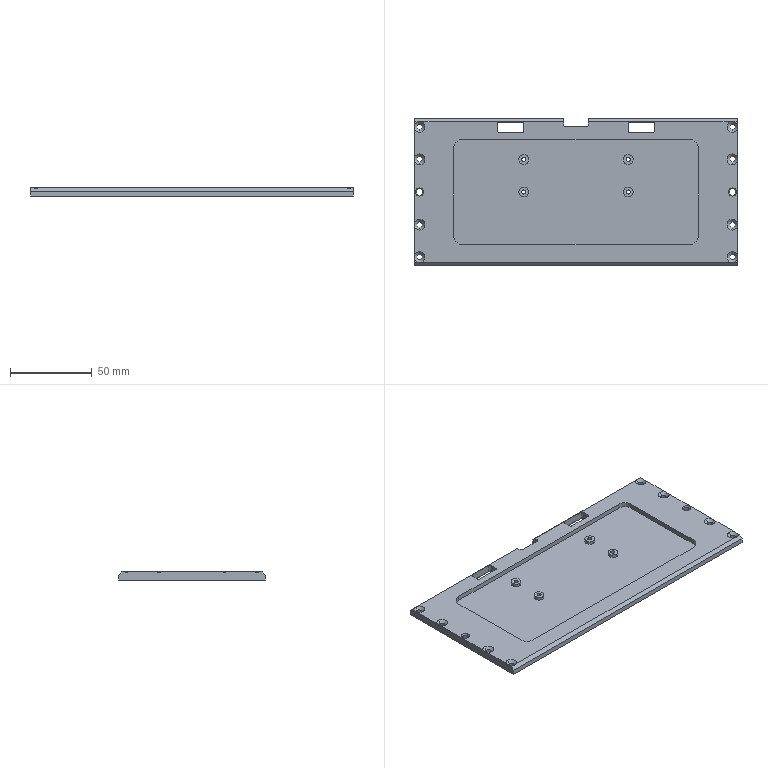NC program | NX | posted with a generic post | part box 198 x 90 x 5 mm
Lines 7363 to 7766 of 7766:
(CUTTERCOMP17 , TOOL : D2)
N14634 T17 M6
N14636 G54
N14638 G17 G0 G90 X-96. Y0. S9500 M3
N14640 G43 Z30. H17
N14642 Z0.5
N14644 G41 G94 G1 X-95.996 Y-0.1 F1100. D17
N14646 G3 X-95.05 Y0. R0.478
N14648 X-95.05 Y0. Z-1.5 I-0.95 J0.
N14650 X-95.05 Y0. Z-3.5 I-0.95 J0.
N14652 X-96. Y-0.95 Z-5. R-0.95
N14654 X-95.05 Y0. R0.95
N14656 X-96. Y-0.95 R-0.95
N14658 X-95.9 Y-0.004 R0.478
N14660 G40
N14662 G1 X-96. Y0.
N14664 G0 Z30.
N14666 X96.
N14668 Z0.5
N14670 G41 G1 X96.004 Y-0.1
N14672 G3 X96.95 Y0. R0.478
N14674 X96.95 Y0. Z-1.5 I-0.95 J0.
N14676 X96.95 Y0. Z-3.5 I-0.95 J0.
N14678 X96. Y-0.95 Z-5. R-0.95
N14680 X96.95 Y0. R0.95
N14682 X96. Y-0.95 R-0.95
N14684 X96.1 Y-0.004 R0.478
N14686 G40
N14688 G1 X96. Y0.
N14690 G0 Z30.
N14692 M5
(ZLEVEL_PROFILE_COPY_1_COPY_COPY_1 , TOOL : D10JING)
N14694 T14 M6
N14696 G54
N14698 G17 G0 G90 X100.622 Y-51.809 S9500 M3
N14700 G43 Z30. H14
N14702 Z-3.525
N14704 G94 G1 Z-4.525 F1000.
N14706 X99.866 Y-50.5
N14708 G3 X99. Y-50. R1.
N14710 G1 X-99. F1200.
N14712 G2 X-104. Y-45. R5.
N14714 G1 Y45.
N14716 G2 X-99. Y50. R5.
N14718 G1 X-7.5
N14720 G2 X-2.5 Y45. R5.
N14722 G1 X2.5
N14724 G2 X7.5 Y50. R5.
N14726 G1 X99.
N14728 G2 X104. Y45. R5.
N14730 G1 Y-45.
N14732 G2 X99. Y-50. R5.
N14734 G1 X-99. Z-4.565
N14736 X-99.49 Y-49.976
N14738 X-99.975 Y-49.904 Z-4.566
N14740 X-100.451 Y-49.785
N14742 X-100.913 Y-49.619
N14744 X-101.357 Y-49.41
N14746 X-101.778 Y-49.157
N14748 X-102.172 Y-48.865
N14750 X-102.536 Y-48.536
N14752 X-102.865 Y-48.172
N14754 X-103.157 Y-47.778
N14756 X-103.41 Y-47.357
N14758 X-103.619 Y-46.913 Z-4.567
N14760 X-103.785 Y-46.451
N14762 X-103.904 Y-45.975
N14764 X-103.976 Y-45.49
N14766 X-104. Y-45.
N14768 X-104.003 Y-40. Z-4.568
N14770 X-104. Y-35. Z-4.569
N14772 Y35. Z-4.583
N14774 X-104.003 Y40. Z-4.584
N14776 X-104. Y45. Z-4.585
N14778 X-103.976 Y45.49
N14780 X-103.904 Y45.975 Z-4.586
N14782 X-103.785 Y46.451
N14784 X-103.619 Y46.913
N14786 X-103.41 Y47.357
N14788 X-103.157 Y47.778
N14790 X-102.865 Y48.172
N14792 X-102.536 Y48.536
N14794 X-102.172 Y48.865
N14796 X-101.778 Y49.157
N14798 X-101.357 Y49.41
N14800 X-100.913 Y49.619 Z-4.587
N14802 X-100.451 Y49.785
N14804 X-99.975 Y49.904
N14806 X-99.49 Y49.976
N14808 X-99. Y50.
N14810 X-7.5 Z-4.606
N14812 X-7.01 Y49.976
N14814 X-6.525 Y49.904
N14816 X-6.049 Y49.785
N14818 X-5.587 Y49.619
N14820 X-5.143 Y49.41
N14822 X-4.722 Y49.157
N14824 X-4.328 Y48.865
N14826 X-3.964 Y48.536
N14828 X-3.635 Y48.172
N14830 X-3.343 Y47.778 Z-4.607
N14832 X-3.09 Y47.357
N14834 X-2.881 Y46.913
N14836 X-2.715 Y46.451
N14838 X-2.596 Y45.975
N14840 X-2.525 Y45.5
N14842 X-2.5 Y45.
N14844 X2.5 Z-4.608
N14846 X2.525 Y45.5
N14848 X2.596 Y45.975
N14850 X2.715 Y46.451
N14852 X2.881 Y46.913 Z-4.609
N14854 X3.09 Y47.357
N14856 X3.343 Y47.778
N14858 X3.635 Y48.172
N14860 X3.964 Y48.536
N14862 X4.328 Y48.865
N14864 X4.722 Y49.157
N14866 X5.143 Y49.41
N14868 X5.587 Y49.619
N14870 X6.049 Y49.785
N14872 X6.525 Y49.904 Z-4.61
N14874 X7.01 Y49.976
N14876 X7.5 Y50.
N14878 X99. Z-4.628
N14880 X99.49 Y49.976 Z-4.629
N14882 X99.975 Y49.904
N14884 X100.451 Y49.785
N14886 X100.913 Y49.619
N14888 X101.357 Y49.41
N14890 X101.778 Y49.157
N14892 X102.172 Y48.865
N14894 X102.536 Y48.536
N14896 X102.865 Y48.172
N14898 X103.157 Y47.778
N14900 X103.41 Y47.357 Z-4.63
N14902 X103.619 Y46.913
N14904 X103.785 Y46.451
N14906 X103.904 Y45.975
N14908 X103.976 Y45.49
N14910 X104. Y45.
N14912 X104.005 Y40.5 Z-4.631
N14914 X104. Y36. Z-4.632
N14916 Y-36. Z-4.647
N14918 X104.005 Y-40.5
N14920 X104. Y-45. Z-4.648
N14922 X103.976 Y-45.49 Z-4.649
N14924 X103.904 Y-45.975
N14926 X103.785 Y-46.451
N14928 X103.619 Y-46.913
N14930 X103.41 Y-47.357
N14932 X103.157 Y-47.778
N14934 X102.865 Y-48.172
N14936 X102.536 Y-48.536
N14938 X102.172 Y-48.865
N14940 X101.778 Y-49.157
N14942 X101.357 Y-49.41 Z-4.65
N14944 X100.913 Y-49.619
N14946 X100.451 Y-49.785
N14948 X99.975 Y-49.904
N14950 X99.49 Y-49.976
N14952 X99. Y-50.
N14954 X-99. Z-4.69
N14956 X-99.49 Y-49.976
N14958 X-99.975 Y-49.904 Z-4.691
N14960 X-100.451 Y-49.785
N14962 X-100.913 Y-49.619
N14964 X-101.357 Y-49.41
N14966 X-101.778 Y-49.157
N14968 X-102.172 Y-48.865
N14970 X-102.536 Y-48.536
N14972 X-102.865 Y-48.172
N14974 X-103.157 Y-47.778
N14976 X-103.41 Y-47.357
N14978 X-103.619 Y-46.913 Z-4.692
N14980 X-103.785 Y-46.451
N14982 X-103.904 Y-45.975
N14984 X-103.976 Y-45.49
N14986 X-104. Y-45.
N14988 X-104.003 Y-40. Z-4.693
N14990 X-104. Y-35. Z-4.694
N14992 Y35. Z-4.708
N14994 X-104.003 Y40. Z-4.709
N14996 X-104. Y45. Z-4.71
N14998 X-103.976 Y45.49
N15000 X-103.904 Y45.975 Z-4.711
N15002 X-103.785 Y46.451
N15004 X-103.619 Y46.913
N15006 X-103.41 Y47.357
N15008 X-103.157 Y47.778
N15010 X-102.865 Y48.172
N15012 X-102.536 Y48.536
N15014 X-102.172 Y48.865
N15016 X-101.778 Y49.157
N15018 X-101.357 Y49.41
N15020 X-100.913 Y49.619 Z-4.712
N15022 X-100.451 Y49.785
N15024 X-99.975 Y49.904
N15026 X-99.49 Y49.976
N15028 X-99. Y50.
N15030 X-7.5 Z-4.731
N15032 X-7.01 Y49.976
N15034 X-6.525 Y49.904
N15036 X-6.049 Y49.785
N15038 X-5.587 Y49.619
N15040 X-5.143 Y49.41
N15042 X-4.722 Y49.157
N15044 X-4.328 Y48.865
N15046 X-3.964 Y48.536
N15048 X-3.635 Y48.172
N15050 X-3.343 Y47.778 Z-4.732
N15052 X-3.09 Y47.357
N15054 X-2.881 Y46.913
N15056 X-2.715 Y46.451
N15058 X-2.596 Y45.975
N15060 X-2.525 Y45.5
N15062 X-2.5 Y45.
N15064 X2.5 Z-4.733
N15066 X2.525 Y45.5
N15068 X2.596 Y45.975
N15070 X2.715 Y46.451
N15072 X2.881 Y46.913 Z-4.734
N15074 X3.09 Y47.357
N15076 X3.343 Y47.778
N15078 X3.635 Y48.172
N15080 X3.964 Y48.536
N15082 X4.328 Y48.865
N15084 X4.722 Y49.157
N15086 X5.143 Y49.41
N15088 X5.587 Y49.619
N15090 X6.049 Y49.785
N15092 X6.525 Y49.904 Z-4.735
N15094 X7.01 Y49.976
N15096 X7.5 Y50.
N15098 X99. Z-4.753
N15100 X99.49 Y49.976 Z-4.754
N15102 X99.975 Y49.904
N15104 X100.451 Y49.785
N15106 X100.913 Y49.619
N15108 X101.357 Y49.41
N15110 X101.778 Y49.157
N15112 X102.172 Y48.865
N15114 X102.536 Y48.536
N15116 X102.865 Y48.172
N15118 X103.157 Y47.778
N15120 X103.41 Y47.357 Z-4.755
N15122 X103.619 Y46.913
N15124 X103.785 Y46.451
N15126 X103.904 Y45.975
N15128 X103.976 Y45.49
N15130 X104. Y45.
N15132 X104.005 Y40.5 Z-4.756
N15134 X104. Y36. Z-4.757
N15136 Y-36. Z-4.772
N15138 X104.005 Y-40.5
N15140 X104. Y-45. Z-4.773
N15142 X103.976 Y-45.49 Z-4.774
N15144 X103.904 Y-45.975
N15146 X103.785 Y-46.451
N15148 X103.619 Y-46.913
N15150 X103.41 Y-47.357
N15152 X103.157 Y-47.778
N15154 X102.865 Y-48.172
N15156 X102.536 Y-48.536
N15158 X102.172 Y-48.865
N15160 X101.778 Y-49.157
N15162 X101.357 Y-49.41 Z-4.775
N15164 X100.913 Y-49.619
N15166 X100.451 Y-49.785
N15168 X99.975 Y-49.904
N15170 X99.49 Y-49.976
N15172 X99. Y-50.
N15174 X-99. Z-4.815
N15176 X-99.49 Y-49.976
N15178 X-99.975 Y-49.904 Z-4.816
N15180 X-100.451 Y-49.785
N15182 X-100.913 Y-49.619
N15184 X-101.357 Y-49.41
N15186 X-101.778 Y-49.157
N15188 X-102.172 Y-48.865
N15190 X-102.536 Y-48.536
N15192 X-102.865 Y-48.172
N15194 X-103.157 Y-47.778
N15196 X-103.41 Y-47.357
N15198 X-103.619 Y-46.913 Z-4.817
N15200 X-103.785 Y-46.451
N15202 X-103.904 Y-45.975
N15204 X-103.976 Y-45.49
N15206 X-104. Y-45.
N15208 X-104.003 Y-40. Z-4.818
N15210 X-104. Y-35. Z-4.819
N15212 Y35. Z-4.833
N15214 X-104.003 Y40. Z-4.834
N15216 X-104. Y45. Z-4.835
N15218 X-103.976 Y45.49
N15220 X-103.904 Y45.975 Z-4.836
N15222 X-103.785 Y46.451
N15224 X-103.619 Y46.913
N15226 X-103.41 Y47.357
N15228 X-103.157 Y47.778
N15230 X-102.865 Y48.172
N15232 X-102.536 Y48.536
N15234 X-102.172 Y48.865
N15236 X-101.778 Y49.157
N15238 X-101.357 Y49.41
N15240 X-100.913 Y49.619 Z-4.837
N15242 X-100.451 Y49.785
N15244 X-99.975 Y49.904
N15246 X-99.49 Y49.976
N15248 X-99. Y50.
N15250 X-7.5 Z-4.856
N15252 X-7.01 Y49.976
N15254 X-6.525 Y49.904
N15256 X-6.049 Y49.785
N15258 X-5.587 Y49.619
N15260 X-5.143 Y49.41
N15262 X-4.722 Y49.157
N15264 X-4.328 Y48.865
N15266 X-3.964 Y48.536
N15268 X-3.635 Y48.172
N15270 X-3.343 Y47.778 Z-4.857
N15272 X-3.09 Y47.357
N15274 X-2.881 Y46.913
N15276 X-2.715 Y46.451
N15278 X-2.596 Y45.975
N15280 X-2.525 Y45.5
N15282 X-2.5 Y45.
N15284 X2.5 Z-4.858
N15286 X2.525 Y45.5
N15288 X2.596 Y45.975
N15290 X2.715 Y46.451
N15292 X2.881 Y46.913 Z-4.859
N15294 X3.09 Y47.357
N15296 X3.343 Y47.778
N15298 X3.635 Y48.172
N15300 X3.964 Y48.536
N15302 X4.328 Y48.865
N15304 X4.722 Y49.157
N15306 X5.143 Y49.41
N15308 X5.587 Y49.619
N15310 X6.049 Y49.785
N15312 X6.525 Y49.904 Z-4.86
N15314 X7.01 Y49.976
N15316 X7.5 Y50.
N15318 X99. Z-4.878
N15320 X99.49 Y49.976 Z-4.879
N15322 X99.975 Y49.904
N15324 X100.451 Y49.785
N15326 X100.913 Y49.619
N15328 X101.357 Y49.41
N15330 X101.778 Y49.157
N15332 X102.172 Y48.865
N15334 X102.536 Y48.536
N15336 X102.865 Y48.172
N15338 X103.157 Y47.778
N15340 X103.41 Y47.357 Z-4.88
N15342 X103.619 Y46.913
N15344 X103.785 Y46.451
N15346 X103.904 Y45.975
N15348 X103.976 Y45.49
N15350 X104. Y45.
N15352 X104.005 Y40.5 Z-4.881
N15354 X104. Y36. Z-4.882
N15356 Y-36. Z-4.897
N15358 X104.005 Y-40.5
N15360 X104. Y-45. Z-4.898
N15362 X103.976 Y-45.49 Z-4.899
N15364 X103.904 Y-45.975
N15366 X103.785 Y-46.451
N15368 X103.619 Y-46.913
N15370 X103.41 Y-47.357
N15372 X103.157 Y-47.778
N15374 X102.865 Y-48.172
N15376 X102.536 Y-48.536
N15378 X102.172 Y-48.865
N15380 X101.778 Y-49.157
N15382 X101.357 Y-49.41 Z-4.9
N15384 X100.913 Y-49.619
N15386 X100.451 Y-49.785
N15388 X99.975 Y-49.904
N15390 X99.49 Y-49.976
N15392 X99. Y-50.
N15394 X-99.
N15396 G2 X-104. Y-45. R5.
N15398 G1 Y45.
N15400 G2 X-99. Y50. R5.
N15402 G1 X-7.5
N15404 G2 X-2.5 Y45. R5.
N15406 G1 X2.5
N15408 G2 X7.5 Y50. R5.
N15410 G1 X99.
N15412 G2 X104. Y45. R5.
N15414 G1 Y-45.
N15416 G2 X99. Y-50. R5.
N15418 G3 X98.134 Y-50.5 R1.
N15420 G1 X97.268 Y-52.
N15422 Z-3.9
N15424 G0 Z30.
N15426 M5
N15428 M2